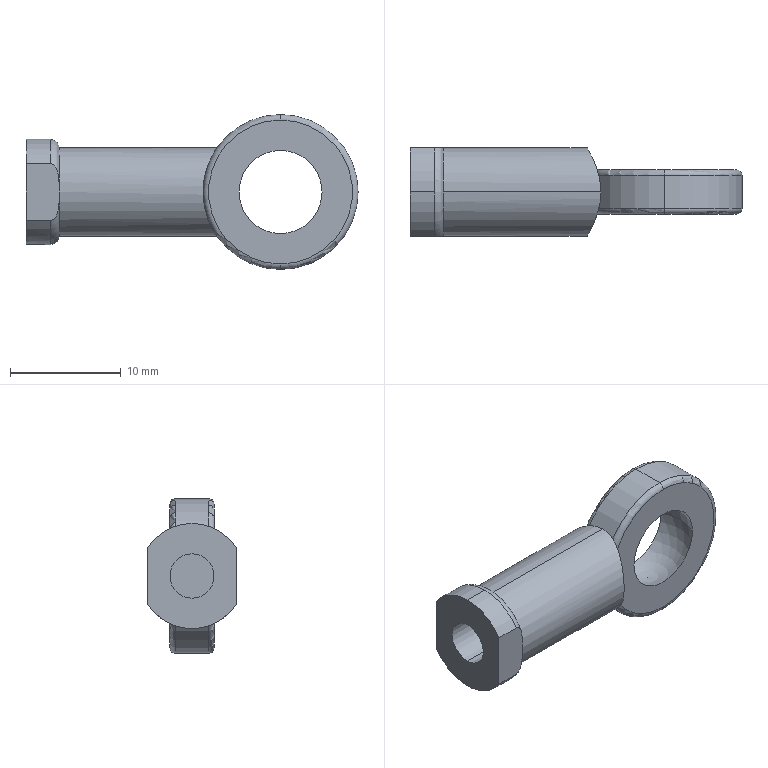Part | SolidWorks | features Fillet 3, ICE 3, Extrusion 1, RevCut 1 | 2 solids | 25 faces | box 30 x 8 x 14 mm | volume 1138 mm3 | cylinder 10 | torus 7 | plane 6 | sphere 2 | commonest cylinder face diameters 9.5 x3 14 x3 4 x2 8 x2
STEP:
#1=CARTESIAN_POINT('',(-3.75,0.,0.));
#2=VERTEX_POINT('',#1);
#3=CARTESIAN_POINT('',(3.75,0.,0.));
#4=VERTEX_POINT('',#3);
#5=CARTESIAN_POINT('',(0.,0.,0.));
#6=DIRECTION('',(0.,-1.,0.));
#7=DIRECTION('',(0.,0.,1.));
#8=AXIS2_PLACEMENT_3D('',#5,#6,#7);
#9=CIRCLE('',#8,3.75);
#10=EDGE_CURVE('',#2,#4,#9,.T.);
#11=ORIENTED_EDGE('',*,*,#10,.T.);
#12=CARTESIAN_POINT('',(3.75,4.,0.));
#13=VERTEX_POINT('',#12);
#14=CARTESIAN_POINT('',(0.,2.,0.));
#15=DIRECTION('',(0.,0.,1.));
#16=DIRECTION('',(1.,0.,0.));
#17=AXIS2_PLACEMENT_3D('',#14,#15,#16);
#18=CIRCLE('',#17,4.25);
#19=EDGE_CURVE('',#4,#13,#18,.T.);
#20=ORIENTED_EDGE('',*,*,#19,.T.);
#21=CARTESIAN_POINT('',(-3.75,4.,0.));
#22=VERTEX_POINT('',#21);
#23=CARTESIAN_POINT('',(0.,4.,0.));
#24=DIRECTION('',(0.,-1.,0.));
#25=DIRECTION('',(0.,0.,1.));
#26=AXIS2_PLACEMENT_3D('',#23,#24,#25);
#27=CIRCLE('',#26,3.75);
#28=EDGE_CURVE('',#22,#13,#27,.T.);
#29=ORIENTED_EDGE('',*,*,#28,.F.);
#30=CARTESIAN_POINT('',(0.,2.,0.));
#31=DIRECTION('',(0.,0.,-1.));
#32=DIRECTION('',(-1.,0.,0.));
#33=AXIS2_PLACEMENT_3D('',#30,#31,#32);
#34=CIRCLE('',#33,4.25);
#35=EDGE_CURVE('',#2,#22,#34,.T.);
#36=ORIENTED_EDGE('',*,*,#35,.F.);
#37=EDGE_LOOP('',(#11,#20,#29,#36));
#38=FACE_OUTER_BOUND('',#37,.T.);
#39=CARTESIAN_POINT('',(0.,2.,0.));
#40=DIRECTION('',(0.,0.,1.));
#41=DIRECTION('',(-1.,0.,0.));
#42=AXIS2_PLACEMENT_3D('',#39,#40,#41);
#43=SPHERICAL_SURFACE('',#42,4.25);
#44=ADVANCED_FACE('',(#38),#43,.F.);
#45=CARTESIAN_POINT('',(0.,3.5,-7.));
#46=VERTEX_POINT('',#45);
#47=CARTESIAN_POINT('',(0.,3.5,7.));
#48=VERTEX_POINT('',#47);
#49=CARTESIAN_POINT('',(0.,3.5,0.));
#50=DIRECTION('',(0.,-1.,0.));
#51=DIRECTION('',(0.,0.,1.));
#52=AXIS2_PLACEMENT_3D('',#49,#50,#51);
#53=CIRCLE('',#52,7.);
#54=EDGE_CURVE('',#46,#48,#53,.T.);
#55=ORIENTED_EDGE('',*,*,#54,.F.);
#56=CARTESIAN_POINT('',(0.,4.,-6.5));
#57=VERTEX_POINT('',#56);
#58=CARTESIAN_POINT('',(0.,3.5,-6.5));
#59=DIRECTION('',(1.,0.,0.));
#60=DIRECTION('',(0.,0.,-1.));
#61=AXIS2_PLACEMENT_3D('',#58,#59,#60);
#62=CIRCLE('',#61,0.5);
#63=EDGE_CURVE('',#46,#57,#62,.T.);
#64=ORIENTED_EDGE('',*,*,#63,.T.);
#65=CARTESIAN_POINT('',(0.,4.,6.5));
#66=VERTEX_POINT('',#65);
#67=CARTESIAN_POINT('',(0.,4.,0.));
#68=DIRECTION('',(0.,1.,0.));
#69=DIRECTION('',(0.,0.,1.));
#70=AXIS2_PLACEMENT_3D('',#67,#68,#69);
#71=CIRCLE('',#70,6.5);
#72=EDGE_CURVE('',#66,#57,#71,.T.);
#73=ORIENTED_EDGE('',*,*,#72,.F.);
#74=CARTESIAN_POINT('',(0.,3.5,6.5));
#75=DIRECTION('',(-1.,0.,0.));
#76=DIRECTION('',(0.,0.,1.));
#77=AXIS2_PLACEMENT_3D('',#74,#75,#76);
#78=CIRCLE('',#77,0.5);
#79=EDGE_CURVE('',#48,#66,#78,.T.);
#80=ORIENTED_EDGE('',*,*,#79,.F.);
#81=EDGE_LOOP('',(#55,#64,#73,#80));
#82=FACE_OUTER_BOUND('',#81,.T.);
#83=CARTESIAN_POINT('',(0.,3.5,0.));
#84=DIRECTION('',(0.,1.,0.));
#85=DIRECTION('',(0.,0.,1.));
#86=AXIS2_PLACEMENT_3D('',#83,#84,#85);
#87=TOROIDAL_SURFACE('',#86,6.5,0.5);
#88=ADVANCED_FACE('',(#82),#87,.T.);
#89=CARTESIAN_POINT('',(0.,0.,-6.5));
#90=VERTEX_POINT('',#89);
#91=CARTESIAN_POINT('',(0.,0.,6.5));
#92=VERTEX_POINT('',#91);
#93=CARTESIAN_POINT('',(0.,0.,0.));
#94=DIRECTION('',(0.,-1.,0.));
#95=DIRECTION('',(0.,0.,1.));
#96=AXIS2_PLACEMENT_3D('',#93,#94,#95);
#97=CIRCLE('',#96,6.5);
#98=EDGE_CURVE('',#90,#92,#97,.T.);
#99=ORIENTED_EDGE('',*,*,#98,.F.);
#100=CARTESIAN_POINT('',(0.,0.5,-7.));
#101=VERTEX_POINT('',#100);
#102=CARTESIAN_POINT('',(0.,0.5,-6.5));
#103=DIRECTION('',(1.,0.,0.));
#104=DIRECTION('',(0.,0.,-1.));
#105=AXIS2_PLACEMENT_3D('',#102,#103,#104);
#106=CIRCLE('',#105,0.5);
#107=EDGE_CURVE('',#90,#101,#106,.T.);
#108=ORIENTED_EDGE('',*,*,#107,.T.);
#109=CARTESIAN_POINT('',(0.,0.5,7.));
#110=VERTEX_POINT('',#109);
#111=CARTESIAN_POINT('',(0.,0.5,0.));
#112=DIRECTION('',(0.,1.,0.));
#113=DIRECTION('',(0.,0.,1.));
#114=AXIS2_PLACEMENT_3D('',#111,#112,#113);
#115=CIRCLE('',#114,7.);
#116=EDGE_CURVE('',#110,#101,#115,.T.);
#117=ORIENTED_EDGE('',*,*,#116,.F.);
#118=CARTESIAN_POINT('',(0.,0.5,6.5));
#119=DIRECTION('',(-1.,0.,0.));
#120=DIRECTION('',(0.,0.,1.));
#121=AXIS2_PLACEMENT_3D('',#118,#119,#120);
#122=CIRCLE('',#121,0.5);
#123=EDGE_CURVE('',#92,#110,#122,.T.);
#124=ORIENTED_EDGE('',*,*,#123,.F.);
#125=EDGE_LOOP('',(#99,#108,#117,#124));
#126=FACE_OUTER_BOUND('',#125,.T.);
#127=CARTESIAN_POINT('',(0.,0.5,0.));
#128=DIRECTION('',(0.,1.,0.));
#129=DIRECTION('',(0.,0.,1.));
#130=AXIS2_PLACEMENT_3D('',#127,#128,#129);
#131=TOROIDAL_SURFACE('',#130,6.5,0.5);
#132=ADVANCED_FACE('',(#126),#131,.T.);
#133=ORIENTED_EDGE('',*,*,#54,.T.);
#134=CARTESIAN_POINT('',(0.,4.,7.));
#135=DIRECTION('',(0.,-1.,0.));
#136=VECTOR('',#135,1000.);
#137=LINE('',#134,#136);
#138=EDGE_CURVE('',#48,#110,#137,.T.);
#139=ORIENTED_EDGE('',*,*,#138,.T.);
#140=ORIENTED_EDGE('',*,*,#116,.T.);
#141=CARTESIAN_POINT('',(0.,4.,-7.));
#142=DIRECTION('',(0.,-1.,0.));
#143=VECTOR('',#142,1000.);
#144=LINE('',#141,#143);
#145=EDGE_CURVE('',#46,#101,#144,.T.);
#146=ORIENTED_EDGE('',*,*,#145,.F.);
#147=EDGE_LOOP('',(#133,#139,#140,#146));
#148=FACE_OUTER_BOUND('',#147,.T.);
#149=CARTESIAN_POINT('',(0.,4.,0.));
#150=DIRECTION('',(0.,-1.,0.));
#151=DIRECTION('',(0.,0.,-1.));
#152=AXIS2_PLACEMENT_3D('',#149,#150,#151);
#153=CYLINDRICAL_SURFACE('',#152,7.);
#154=ADVANCED_FACE('',(#148),#153,.T.);
#155=ORIENTED_EDGE('',*,*,#28,.T.);
#156=CARTESIAN_POINT('',(0.,4.,0.));
#157=DIRECTION('',(0.,-1.,0.));
#158=DIRECTION('',(0.,0.,1.));
#159=AXIS2_PLACEMENT_3D('',#156,#157,#158);
#160=CIRCLE('',#159,3.75);
#161=EDGE_CURVE('',#13,#22,#160,.T.);
#162=ORIENTED_EDGE('',*,*,#161,.T.);
#163=EDGE_LOOP('',(#155,#162));
#164=FACE_BOUND('',#163,.T.);
#165=ORIENTED_EDGE('',*,*,#72,.T.);
#166=CARTESIAN_POINT('',(0.,4.,0.));
#167=DIRECTION('',(0.,1.,0.));
#168=DIRECTION('',(0.,0.,1.));
#169=AXIS2_PLACEMENT_3D('',#166,#167,#168);
#170=CIRCLE('',#169,6.5);
#171=EDGE_CURVE('',#57,#66,#170,.T.);
#172=ORIENTED_EDGE('',*,*,#171,.T.);
#173=EDGE_LOOP('',(#165,#172));
#174=FACE_OUTER_BOUND('',#173,.T.);
#175=CARTESIAN_POINT('',(0.,4.,0.));
#176=DIRECTION('',(0.,1.,0.));
#177=DIRECTION('',(0.,0.,1.));
#178=AXIS2_PLACEMENT_3D('',#175,#176,#177);
#179=PLANE('',#178);
#180=ADVANCED_FACE('',(#164,#174),#179,.T.);
#181=ORIENTED_EDGE('',*,*,#10,.F.);
#182=CARTESIAN_POINT('',(0.,0.,0.));
#183=DIRECTION('',(0.,-1.,0.));
#184=DIRECTION('',(0.,0.,1.));
#185=AXIS2_PLACEMENT_3D('',#182,#183,#184);
#186=CIRCLE('',#185,3.75);
#187=EDGE_CURVE('',#4,#2,#186,.T.);
#188=ORIENTED_EDGE('',*,*,#187,.F.);
#189=EDGE_LOOP('',(#181,#188));
#190=FACE_BOUND('',#189,.T.);
#191=CARTESIAN_POINT('',(0.,0.,0.));
#192=DIRECTION('',(0.,-1.,0.));
#193=DIRECTION('',(0.,0.,1.));
#194=AXIS2_PLACEMENT_3D('',#191,#192,#193);
#195=CIRCLE('',#194,6.5);
#196=EDGE_CURVE('',#92,#90,#195,.T.);
#197=ORIENTED_EDGE('',*,*,#196,.T.);
#198=ORIENTED_EDGE('',*,*,#98,.T.);
#199=EDGE_LOOP('',(#197,#198));
#200=FACE_OUTER_BOUND('',#199,.T.);
#201=CARTESIAN_POINT('',(0.,0.,0.));
#202=DIRECTION('',(0.,1.,0.));
#203=DIRECTION('',(0.,0.,1.));
#204=AXIS2_PLACEMENT_3D('',#201,#202,#203);
#205=PLANE('',#204);
#206=ADVANCED_FACE('',(#190,#200),#205,.F.);
#207=ORIENTED_EDGE('',*,*,#138,.F.);
#208=CARTESIAN_POINT('',(0.,3.5,0.));
#209=DIRECTION('',(0.,-1.,0.));
#210=DIRECTION('',(0.,0.,1.));
#211=AXIS2_PLACEMENT_3D('',#208,#209,#210);
#212=CIRCLE('',#211,7.);
#213=EDGE_CURVE('',#48,#46,#212,.T.);
#214=ORIENTED_EDGE('',*,*,#213,.T.);
#215=ORIENTED_EDGE('',*,*,#145,.T.);
#216=CARTESIAN_POINT('',(0.,0.5,0.));
#217=DIRECTION('',(0.,1.,0.));
#218=DIRECTION('',(0.,0.,1.));
#219=AXIS2_PLACEMENT_3D('',#216,#217,#218);
#220=CIRCLE('',#219,7.);
#221=EDGE_CURVE('',#101,#110,#220,.T.);
#222=ORIENTED_EDGE('',*,*,#221,.T.);
#223=EDGE_LOOP('',(#207,#214,#215,#222));
#224=FACE_OUTER_BOUND('',#223,.T.);
#225=CARTESIAN_POINT('',(0.,4.,0.));
#226=DIRECTION('',(0.,-1.,0.));
#227=DIRECTION('',(0.,0.,-1.));
#228=AXIS2_PLACEMENT_3D('',#225,#226,#227);
#229=CYLINDRICAL_SURFACE('',#228,7.);
#230=ADVANCED_FACE('',(#224),#229,.T.);
#231=ORIENTED_EDGE('',*,*,#107,.F.);
#232=ORIENTED_EDGE('',*,*,#196,.F.);
#233=ORIENTED_EDGE('',*,*,#123,.T.);
#234=ORIENTED_EDGE('',*,*,#221,.F.);
#235=EDGE_LOOP('',(#231,#232,#233,#234));
#236=FACE_OUTER_BOUND('',#235,.T.);
#237=CARTESIAN_POINT('',(0.,0.5,0.));
#238=DIRECTION('',(0.,1.,0.));
#239=DIRECTION('',(0.,0.,1.));
#240=AXIS2_PLACEMENT_3D('',#237,#238,#239);
#241=TOROIDAL_SURFACE('',#240,6.5,0.5);
#242=ADVANCED_FACE('',(#236),#241,.T.);
#243=ORIENTED_EDGE('',*,*,#63,.F.);
#244=ORIENTED_EDGE('',*,*,#213,.F.);
#245=ORIENTED_EDGE('',*,*,#79,.T.);
#246=ORIENTED_EDGE('',*,*,#171,.F.);
#247=EDGE_LOOP('',(#243,#244,#245,#246));
#248=FACE_OUTER_BOUND('',#247,.T.);
#249=CARTESIAN_POINT('',(0.,3.5,0.));
#250=DIRECTION('',(0.,1.,0.));
#251=DIRECTION('',(0.,0.,1.));
#252=AXIS2_PLACEMENT_3D('',#249,#250,#251);
#253=TOROIDAL_SURFACE('',#252,6.5,0.5);
#254=ADVANCED_FACE('',(#248),#253,.T.);
#255=ORIENTED_EDGE('',*,*,#19,.F.);
#256=ORIENTED_EDGE('',*,*,#187,.T.);
#257=ORIENTED_EDGE('',*,*,#35,.T.);
#258=ORIENTED_EDGE('',*,*,#161,.F.);
#259=EDGE_LOOP('',(#255,#256,#257,#258));
#260=FACE_OUTER_BOUND('',#259,.T.);
#261=CARTESIAN_POINT('',(0.,2.,0.));
#262=DIRECTION('',(0.,0.,1.));
#263=DIRECTION('',(-1.,0.,0.));
#264=AXIS2_PLACEMENT_3D('',#261,#262,#263);
#265=SPHERICAL_SURFACE('',#264,4.25);
#266=ADVANCED_FACE('',(#260),#265,.F.);
#267=CLOSED_SHELL('',(#44,#88,#132,#154,#180,#206,#230,#242,#254,#266));
#268=MANIFOLD_SOLID_BREP('',#267);
#269=CARTESIAN_POINT('',(-13.,2.,-2.));
#270=VERTEX_POINT('',#269);
#271=CARTESIAN_POINT('',(-13.,2.,2.));
#272=VERTEX_POINT('',#271);
#273=CARTESIAN_POINT('',(-13.,2.,0.));
#274=DIRECTION('',(-1.,0.,0.));
#275=DIRECTION('',(0.,0.,1.));
#276=AXIS2_PLACEMENT_3D('',#273,#274,#275);
#277=CIRCLE('',#276,2.);
#278=EDGE_CURVE('',#270,#272,#277,.T.);
#279=ORIENTED_EDGE('',*,*,#278,.F.);
#280=CARTESIAN_POINT('',(-23.,2.,-2.));
#281=VERTEX_POINT('',#280);
#282=CARTESIAN_POINT('',(-13.,2.,-2.));
#283=DIRECTION('',(-1.,0.,0.));
#284=VECTOR('',#283,1000.);
#285=LINE('',#282,#284);
#286=EDGE_CURVE('',#270,#281,#285,.T.);
#287=ORIENTED_EDGE('',*,*,#286,.T.);
#288=CARTESIAN_POINT('',(-23.,2.,2.));
#289=VERTEX_POINT('',#288);
#290=CARTESIAN_POINT('',(-23.,2.,0.));
#291=DIRECTION('',(-1.,0.,0.));
#292=DIRECTION('',(0.,0.,1.));
#293=AXIS2_PLACEMENT_3D('',#290,#291,#292);
#294=CIRCLE('',#293,2.);
#295=EDGE_CURVE('',#281,#289,#294,.T.);
#296=ORIENTED_EDGE('',*,*,#295,.T.);
#297=CARTESIAN_POINT('',(-13.,2.,2.));
#298=DIRECTION('',(-1.,0.,0.));
#299=VECTOR('',#298,1000.);
#300=LINE('',#297,#299);
#301=EDGE_CURVE('',#272,#289,#300,.T.);
#302=ORIENTED_EDGE('',*,*,#301,.F.);
#303=EDGE_LOOP('',(#279,#287,#296,#302));
#304=FACE_OUTER_BOUND('',#303,.T.);
#305=CARTESIAN_POINT('',(-13.,2.,0.));
#306=DIRECTION('',(-1.,0.,0.));
#307=DIRECTION('',(0.,0.,1.));
#308=AXIS2_PLACEMENT_3D('',#305,#306,#307);
#309=CYLINDRICAL_SURFACE('',#308,2.);
#310=ADVANCED_FACE('',(#304),#309,.F.);
#311=CARTESIAN_POINT('',(-20.798,2.,-4.75));
#312=VERTEX_POINT('',#311);
#313=CARTESIAN_POINT('',(-20.798,-2.,-2.562));
#314=VERTEX_POINT('',#313);
#315=CARTESIAN_POINT('',(-20.798,2.,0.));
#316=DIRECTION('',(-1.,0.,0.));
#317=DIRECTION('',(0.,0.,-1.));
#318=AXIS2_PLACEMENT_3D('',#315,#316,#317);
#319=CIRCLE('',#318,4.75);
#320=EDGE_CURVE('',#312,#314,#319,.T.);
#321=ORIENTED_EDGE('',*,*,#320,.F.);
#322=CARTESIAN_POINT('',(-20.,2.,-4.));
#323=VERTEX_POINT('',#322);
#324=CARTESIAN_POINT('',(-20.798,2.,-3.95));
#325=DIRECTION('',(0.,-1.,0.));
#326=DIRECTION('',(0.,0.,-1.));
#327=AXIS2_PLACEMENT_3D('',#324,#325,#326);
#328=CIRCLE('',#327,0.8);
#329=EDGE_CURVE('',#312,#323,#328,.T.);
#330=ORIENTED_EDGE('',*,*,#329,.T.);
#331=CARTESIAN_POINT('',(-20.,-2.,0.));
#332=VERTEX_POINT('',#331);
#333=CARTESIAN_POINT('',(-20.,2.,0.));
#334=DIRECTION('',(-1.,0.,0.));
#335=DIRECTION('',(0.,0.,1.));
#336=AXIS2_PLACEMENT_3D('',#333,#334,#335);
#337=CIRCLE('',#336,4.);
#338=EDGE_CURVE('',#323,#332,#337,.T.);
#339=ORIENTED_EDGE('',*,*,#338,.T.);
#340=CARTESIAN_POINT('',(-20.798,-2.,-2.562));
#341=CARTESIAN_POINT('',(-20.675,-2.,-2.562));
#342=CARTESIAN_POINT('',(-20.558,-2.,-2.506));
#343=CARTESIAN_POINT('',(-20.376,-2.,-2.346));
#344=CARTESIAN_POINT('',(-20.306,-2.,-2.243));
#345=CARTESIAN_POINT('',(-20.197,-2.,-2.027));
#346=CARTESIAN_POINT('',(-20.157,-2.,-1.911));
#347=CARTESIAN_POINT('',(-20.096,-2.,-1.678));
#348=CARTESIAN_POINT('',(-20.074,-2.,-1.56));
#349=CARTESIAN_POINT('',(-20.025,-2.,-1.204));
#350=CARTESIAN_POINT('',(-20.013,-2.,-0.9634));
#351=CARTESIAN_POINT('',(-20.001,-2.,-0.4818));
#352=CARTESIAN_POINT('',(-20.,-2.,-0.2409));
#353=CARTESIAN_POINT('',(-20.,-2.,0.));
#354=B_SPLINE_CURVE_WITH_KNOTS('',3,(#340,#341,#342,#343,#344,#345,#346,#347,#348,#349,#350,#351,#352,#353),.UNSPECIFIED.,.F.,.F.,(4,2,2,2,2,2,4),(0.,0.0003642,0.0007284,0.001093,0.001457,0.002185,0.002914),.UNSPECIFIED.);
#355=EDGE_CURVE('',#314,#332,#354,.T.);
#356=ORIENTED_EDGE('',*,*,#355,.F.);
#357=EDGE_LOOP('',(#321,#330,#339,#356));
#358=FACE_OUTER_BOUND('',#357,.T.);
#359=CARTESIAN_POINT('',(-20.798,2.,0.));
#360=DIRECTION('',(1.,0.,0.));
#361=DIRECTION('',(0.,0.,-1.));
#362=AXIS2_PLACEMENT_3D('',#359,#360,#361);
#363=TOROIDAL_SURFACE('',#362,3.95,0.8);
#364=ADVANCED_FACE('',(#358),#363,.T.);
#365=CARTESIAN_POINT('',(-20.798,-2.,2.562));
#366=VERTEX_POINT('',#365);
#367=CARTESIAN_POINT('',(-20.798,2.,4.75));
#368=VERTEX_POINT('',#367);
#369=CARTESIAN_POINT('',(-20.798,2.,0.));
#370=DIRECTION('',(-1.,0.,0.));
#371=DIRECTION('',(0.,0.,-1.));
#372=AXIS2_PLACEMENT_3D('',#369,#370,#371);
#373=CIRCLE('',#372,4.75);
#374=EDGE_CURVE('',#366,#368,#373,.T.);
#375=ORIENTED_EDGE('',*,*,#374,.T.);
#376=CARTESIAN_POINT('',(-23.,2.,4.75));
#377=VERTEX_POINT('',#376);
#378=CARTESIAN_POINT('',(-20.,2.,4.75));
#379=DIRECTION('',(-1.,0.,0.));
#380=VECTOR('',#379,1000.);
#381=LINE('',#378,#380);
#382=EDGE_CURVE('',#368,#377,#381,.T.);
#383=ORIENTED_EDGE('',*,*,#382,.T.);
#384=CARTESIAN_POINT('',(-23.,-2.,2.562));
#385=VERTEX_POINT('',#384);
#386=CARTESIAN_POINT('',(-23.,2.,0.));
#387=DIRECTION('',(-1.,0.,0.));
#388=DIRECTION('',(0.,0.,1.));
#389=AXIS2_PLACEMENT_3D('',#386,#387,#388);
#390=CIRCLE('',#389,4.75);
#391=EDGE_CURVE('',#385,#377,#390,.T.);
#392=ORIENTED_EDGE('',*,*,#391,.F.);
#393=CARTESIAN_POINT('',(-20.,-2.,2.562));
#394=DIRECTION('',(-1.,0.,0.));
#395=VECTOR('',#394,1000.);
#396=LINE('',#393,#395);
#397=EDGE_CURVE('',#366,#385,#396,.T.);
#398=ORIENTED_EDGE('',*,*,#397,.F.);
#399=EDGE_LOOP('',(#375,#383,#392,#398));
#400=FACE_OUTER_BOUND('',#399,.T.);
#401=CARTESIAN_POINT('',(-20.,2.,0.));
#402=DIRECTION('',(-1.,0.,0.));
#403=DIRECTION('',(0.,0.,1.));
#404=AXIS2_PLACEMENT_3D('',#401,#402,#403);
#405=CYLINDRICAL_SURFACE('',#404,4.75);
#406=ADVANCED_FACE('',(#400),#405,.T.);
#407=CARTESIAN_POINT('',(-20.,2.,4.));
#408=VERTEX_POINT('',#407);
#409=CARTESIAN_POINT('',(-20.,6.,0.));
#410=VERTEX_POINT('',#409);
#411=CARTESIAN_POINT('',(-20.,2.,0.));
#412=DIRECTION('',(-1.,0.,0.));
#413=DIRECTION('',(0.,0.,1.));
#414=AXIS2_PLACEMENT_3D('',#411,#412,#413);
#415=CIRCLE('',#414,4.);
#416=EDGE_CURVE('',#408,#410,#415,.T.);
#417=ORIENTED_EDGE('',*,*,#416,.F.);
#418=CARTESIAN_POINT('',(-5.745,2.,4.));
#419=VERTEX_POINT('',#418);
#420=CARTESIAN_POINT('',(-23.,2.,4.));
#421=DIRECTION('',(1.,0.,0.));
#422=VECTOR('',#421,1000.);
#423=LINE('',#420,#422);
#424=EDGE_CURVE('',#408,#419,#423,.T.);
#425=ORIENTED_EDGE('',*,*,#424,.T.);
#426=CARTESIAN_POINT('',(-5.745,2.,-4.));
#427=VERTEX_POINT('',#426);
#428=CARTESIAN_POINT('',(-5.745,2.,4.));
#429=CARTESIAN_POINT('',(-5.745,2.271,4.));
#430=CARTESIAN_POINT('',(-5.764,2.536,3.973));
#431=CARTESIAN_POINT('',(-5.835,3.055,3.868));
#432=CARTESIAN_POINT('',(-5.888,3.31,3.788));
#433=CARTESIAN_POINT('',(-6.075,4.031,3.485));
#434=CARTESIAN_POINT('',(-6.242,4.463,3.193));
#435=CARTESIAN_POINT('',(-6.481,5.005,2.652));
#436=CARTESIAN_POINT('',(-6.56,5.171,2.452));
#437=CARTESIAN_POINT('',(-6.705,5.46,2.024));
#438=CARTESIAN_POINT('',(-6.77,5.583,1.797));
#439=CARTESIAN_POINT('',(-6.879,5.786,1.317));
#440=CARTESIAN_POINT('',(-6.924,5.866,1.059));
#441=CARTESIAN_POINT('',(-6.984,5.972,0.539));
#442=CARTESIAN_POINT('',(-7.,6.,0.2747));
#443=CARTESIAN_POINT('',(-7.,6.,-0.1284));
#444=CARTESIAN_POINT('',(-6.996,5.994,-0.2644));
#445=CARTESIAN_POINT('',(-6.981,5.967,-0.5313));
#446=CARTESIAN_POINT('',(-6.97,5.947,-0.663));
#447=CARTESIAN_POINT('',(-6.925,5.868,-1.053));
#448=CARTESIAN_POINT('',(-6.881,5.789,-1.31));
#449=CARTESIAN_POINT('',(-6.771,5.584,-1.795));
#450=CARTESIAN_POINT('',(-6.705,5.46,-2.023));
#451=CARTESIAN_POINT('',(-6.56,5.17,-2.453));
#452=CARTESIAN_POINT('',(-6.481,5.005,-2.652));
#453=CARTESIAN_POINT('',(-6.322,4.644,-3.013));
#454=CARTESIAN_POINT('',(-6.24,4.445,-3.176));
#455=CARTESIAN_POINT('',(-6.085,4.017,-3.464));
#456=CARTESIAN_POINT('',(-6.013,3.791,-3.586));
#457=CARTESIAN_POINT('',(-5.919,3.432,-3.737));
#458=CARTESIAN_POINT('',(-5.891,3.31,-3.782));
#459=CARTESIAN_POINT('',(-5.84,3.057,-3.86));
#460=CARTESIAN_POINT('',(-5.817,2.927,-3.893));
#461=CARTESIAN_POINT('',(-5.764,2.536,-3.973));
#462=CARTESIAN_POINT('',(-5.745,2.27,-4.));
#463=CARTESIAN_POINT('',(-5.745,2.,-4.));
#464=B_SPLINE_CURVE_WITH_KNOTS('',3,(#428,#429,#430,#431,#432,#433,#434,#435,#436,#437,#438,#439,#440,#441,#442,#443,#444,#445,#446,#447,#448,#449,#450,#451,#452,#453,#454,#455,#456,#457,#458,#459,#460,#461,#462,#463),.UNSPECIFIED.,.F.,.F.,(4,2,2,2,2,2,2,2,2,2,2,2,2,2,2,2,2,4),(0.,0.0007996,0.001599,0.003198,0.003998,0.004798,0.005597,0.006397,0.006797,0.007197,0.007996,0.008796,0.009595,0.0104,0.01119,0.01159,0.01199,0.01279),.UNSPECIFIED.);
#465=EDGE_CURVE('',#419,#427,#464,.T.);
#466=ORIENTED_EDGE('',*,*,#465,.T.);
#467=CARTESIAN_POINT('',(-23.,2.,-4.));
#468=DIRECTION('',(1.,0.,0.));
#469=VECTOR('',#468,1000.);
#470=LINE('',#467,#469);
#471=EDGE_CURVE('',#323,#427,#470,.T.);
#472=ORIENTED_EDGE('',*,*,#471,.F.);
#473=CARTESIAN_POINT('',(-20.,2.,0.));
#474=DIRECTION('',(-1.,0.,0.));
#475=DIRECTION('',(0.,0.,1.));
#476=AXIS2_PLACEMENT_3D('',#473,#474,#475);
#477=CIRCLE('',#476,4.);
#478=EDGE_CURVE('',#410,#323,#477,.T.);
#479=ORIENTED_EDGE('',*,*,#478,.F.);
#480=EDGE_LOOP('',(#417,#425,#466,#472,#479));
#481=FACE_OUTER_BOUND('',#480,.T.);
#482=CARTESIAN_POINT('',(-23.,2.,0.));
#483=DIRECTION('',(1.,0.,0.));
#484=DIRECTION('',(0.,0.,-1.));
#485=AXIS2_PLACEMENT_3D('',#482,#483,#484);
#486=CYLINDRICAL_SURFACE('',#485,4.);
#487=ADVANCED_FACE('',(#481),#486,.T.);
#488=ORIENTED_EDGE('',*,*,#424,.F.);
#489=CARTESIAN_POINT('',(-20.,2.,0.));
#490=DIRECTION('',(-1.,0.,0.));
#491=DIRECTION('',(0.,0.,1.));
#492=AXIS2_PLACEMENT_3D('',#489,#490,#491);
#493=CIRCLE('',#492,4.);
#494=EDGE_CURVE('',#332,#408,#493,.T.);
#495=ORIENTED_EDGE('',*,*,#494,.F.);
#496=ORIENTED_EDGE('',*,*,#338,.F.);
#497=ORIENTED_EDGE('',*,*,#471,.T.);
#498=CARTESIAN_POINT('',(-5.745,2.,-4.));
#499=CARTESIAN_POINT('',(-5.745,1.73,-4.));
#500=CARTESIAN_POINT('',(-5.764,1.463,-3.973));
#501=CARTESIAN_POINT('',(-5.835,0.9435,-3.867));
#502=CARTESIAN_POINT('',(-5.888,0.6879,-3.788));
#503=CARTESIAN_POINT('',(-6.013,0.2078,-3.586));
#504=CARTESIAN_POINT('',(-6.086,-0.01982,-3.462));
#505=CARTESIAN_POINT('',(-6.241,-0.4485,-3.174));
#506=CARTESIAN_POINT('',(-6.322,-0.6451,-3.011));
#507=CARTESIAN_POINT('',(-6.482,-1.006,-2.651));
#508=CARTESIAN_POINT('',(-6.561,-1.172,-2.45));
#509=CARTESIAN_POINT('',(-6.705,-1.46,-2.023));
#510=CARTESIAN_POINT('',(-6.77,-1.583,-1.797));
#511=CARTESIAN_POINT('',(-6.88,-1.787,-1.315));
#512=CARTESIAN_POINT('',(-6.925,-1.867,-1.058));
#513=CARTESIAN_POINT('',(-6.984,-1.972,-0.5385));
#514=CARTESIAN_POINT('',(-7.,-2.,-0.2742));
#515=CARTESIAN_POINT('',(-7.,-2.,0.2646));
#516=CARTESIAN_POINT('',(-6.985,-1.973,0.5333));
#517=CARTESIAN_POINT('',(-6.925,-1.868,1.054));
#518=CARTESIAN_POINT('',(-6.881,-1.788,1.311));
#519=CARTESIAN_POINT('',(-6.771,-1.584,1.795));
#520=CARTESIAN_POINT('',(-6.705,-1.461,2.023));
#521=CARTESIAN_POINT('',(-6.56,-1.17,2.453));
#522=CARTESIAN_POINT('',(-6.481,-1.005,2.652));
#523=CARTESIAN_POINT('',(-6.322,-0.6439,3.012));
#524=CARTESIAN_POINT('',(-6.24,-0.4442,3.177));
#525=CARTESIAN_POINT('',(-6.085,-0.0172,3.464));
#526=CARTESIAN_POINT('',(-6.013,0.2084,3.586));
#527=CARTESIAN_POINT('',(-5.888,0.6864,3.787));
#528=CARTESIAN_POINT('',(-5.835,0.9424,3.867));
#529=CARTESIAN_POINT('',(-5.764,1.463,3.973));
#530=CARTESIAN_POINT('',(-5.745,1.73,4.));
#531=CARTESIAN_POINT('',(-5.745,2.,4.));
#532=B_SPLINE_CURVE_WITH_KNOTS('',3,(#498,#499,#500,#501,#502,#503,#504,#505,#506,#507,#508,#509,#510,#511,#512,#513,#514,#515,#516,#517,#518,#519,#520,#521,#522,#523,#524,#525,#526,#527,#528,#529,#530,#531),.UNSPECIFIED.,.F.,.F.,(4,2,2,2,2,2,2,2,2,2,2,2,2,2,2,2,4),(0.01279,0.01359,0.01439,0.01519,0.01599,0.01678,0.01758,0.01838,0.01918,0.01998,0.02077,0.02157,0.02237,0.02317,0.02397,0.02476,0.02556),.UNSPECIFIED.);
#533=EDGE_CURVE('',#427,#419,#532,.T.);
#534=ORIENTED_EDGE('',*,*,#533,.T.);
#535=EDGE_LOOP('',(#488,#495,#496,#497,#534));
#536=FACE_OUTER_BOUND('',#535,.T.);
#537=CARTESIAN_POINT('',(-23.,2.,0.));
#538=DIRECTION('',(1.,0.,0.));
#539=DIRECTION('',(0.,0.,-1.));
#540=AXIS2_PLACEMENT_3D('',#537,#538,#539);
#541=CYLINDRICAL_SURFACE('',#540,4.);
#542=ADVANCED_FACE('',(#536),#541,.T.);
#543=ORIENTED_EDGE('',*,*,#533,.F.);
#544=ORIENTED_EDGE('',*,*,#465,.F.);
#545=EDGE_LOOP('',(#543,#544));
#546=FACE_OUTER_BOUND('',#545,.T.);
#547=CARTESIAN_POINT('',(0.,4.,0.));
#548=DIRECTION('',(0.,-1.,0.));
#549=DIRECTION('',(0.,0.,-1.));
#550=AXIS2_PLACEMENT_3D('',#547,#548,#549);
#551=CYLINDRICAL_SURFACE('',#550,7.);
#552=ADVANCED_FACE('',(#546),#551,.F.);
#553=CARTESIAN_POINT('',(-23.,-2.,-2.562));
#554=VERTEX_POINT('',#553);
#555=CARTESIAN_POINT('',(-20.,-2.,-2.562));
#556=DIRECTION('',(-1.,0.,0.));
#557=VECTOR('',#556,1000.);
#558=LINE('',#555,#557);
#559=EDGE_CURVE('',#314,#554,#558,.T.);
#560=ORIENTED_EDGE('',*,*,#559,.F.);
#561=ORIENTED_EDGE('',*,*,#355,.T.);
#562=CARTESIAN_POINT('',(-20.,-2.,0.));
#563=CARTESIAN_POINT('',(-20.,-2.,0.2407));
#564=CARTESIAN_POINT('',(-20.001,-2.,0.4815));
#565=CARTESIAN_POINT('',(-20.013,-2.,0.9623));
#566=CARTESIAN_POINT('',(-20.025,-2.,1.202));
#567=CARTESIAN_POINT('',(-20.074,-2.,1.561));
#568=CARTESIAN_POINT('',(-20.096,-2.,1.681));
#569=CARTESIAN_POINT('',(-20.158,-2.,1.914));
#570=CARTESIAN_POINT('',(-20.199,-2.,2.03));
#571=CARTESIAN_POINT('',(-20.307,-2.,2.244));
#572=CARTESIAN_POINT('',(-20.376,-2.,2.346));
#573=CARTESIAN_POINT('',(-20.559,-2.,2.506));
#574=CARTESIAN_POINT('',(-20.675,-2.,2.562));
#575=CARTESIAN_POINT('',(-20.798,-2.,2.562));
#576=B_SPLINE_CURVE_WITH_KNOTS('',3,(#562,#563,#564,#565,#566,#567,#568,#569,#570,#571,#572,#573,#574,#575),.UNSPECIFIED.,.F.,.F.,(4,2,2,2,2,2,4),(0.,0.0007213,0.001443,0.001803,0.002164,0.002524,0.002885),.UNSPECIFIED.);
#577=EDGE_CURVE('',#332,#366,#576,.T.);
#578=ORIENTED_EDGE('',*,*,#577,.T.);
#579=ORIENTED_EDGE('',*,*,#397,.T.);
#580=CARTESIAN_POINT('',(-23.,-2.,2.562));
#581=DIRECTION('',(0.,0.,1.));
#582=VECTOR('',#581,1000.);
#583=LINE('',#580,#582);
#584=EDGE_CURVE('',#554,#385,#583,.T.);
#585=ORIENTED_EDGE('',*,*,#584,.F.);
#586=EDGE_LOOP('',(#560,#561,#578,#579,#585));
#587=FACE_OUTER_BOUND('',#586,.T.);
#588=CARTESIAN_POINT('',(-20.,-2.,2.562));
#589=DIRECTION('',(0.,-1.,0.));
#590=DIRECTION('',(0.,0.,-1.));
#591=AXIS2_PLACEMENT_3D('',#588,#589,#590);
#592=PLANE('',#591);
#593=ADVANCED_FACE('',(#587),#592,.T.);
#594=CARTESIAN_POINT('',(-20.798,6.,2.562));
#595=VERTEX_POINT('',#594);
#596=CARTESIAN_POINT('',(-20.798,6.,2.562));
#597=CARTESIAN_POINT('',(-20.675,6.,2.562));
#598=CARTESIAN_POINT('',(-20.558,6.,2.506));
#599=CARTESIAN_POINT('',(-20.376,6.,2.346));
#600=CARTESIAN_POINT('',(-20.306,6.,2.243));
#601=CARTESIAN_POINT('',(-20.197,6.,2.027));
#602=CARTESIAN_POINT('',(-20.157,6.,1.911));
#603=CARTESIAN_POINT('',(-20.096,6.,1.678));
#604=CARTESIAN_POINT('',(-20.074,6.,1.56));
#605=CARTESIAN_POINT('',(-20.025,6.,1.204));
#606=CARTESIAN_POINT('',(-20.013,6.,0.9634));
#607=CARTESIAN_POINT('',(-20.001,6.,0.4818));
#608=CARTESIAN_POINT('',(-20.,6.,0.2409));
#609=CARTESIAN_POINT('',(-20.,6.,0.));
#610=B_SPLINE_CURVE_WITH_KNOTS('',3,(#596,#597,#598,#599,#600,#601,#602,#603,#604,#605,#606,#607,#608,#609),.UNSPECIFIED.,.F.,.F.,(4,2,2,2,2,2,4),(0.,0.0003642,0.0007284,0.001093,0.001457,0.002185,0.002914),.UNSPECIFIED.);
#611=EDGE_CURVE('',#595,#410,#610,.T.);
#612=ORIENTED_EDGE('',*,*,#611,.T.);
#613=CARTESIAN_POINT('',(-20.798,6.,-2.562));
#614=VERTEX_POINT('',#613);
#615=CARTESIAN_POINT('',(-20.,6.,0.));
#616=CARTESIAN_POINT('',(-20.,6.,-0.2407));
#617=CARTESIAN_POINT('',(-20.001,6.,-0.4815));
#618=CARTESIAN_POINT('',(-20.013,6.,-0.9623));
#619=CARTESIAN_POINT('',(-20.025,6.,-1.202));
#620=CARTESIAN_POINT('',(-20.074,6.,-1.561));
#621=CARTESIAN_POINT('',(-20.096,6.,-1.681));
#622=CARTESIAN_POINT('',(-20.158,6.,-1.914));
#623=CARTESIAN_POINT('',(-20.199,6.,-2.03));
#624=CARTESIAN_POINT('',(-20.307,6.,-2.244));
#625=CARTESIAN_POINT('',(-20.376,6.,-2.346));
#626=CARTESIAN_POINT('',(-20.559,6.,-2.506));
#627=CARTESIAN_POINT('',(-20.675,6.,-2.562));
#628=CARTESIAN_POINT('',(-20.798,6.,-2.562));
#629=B_SPLINE_CURVE_WITH_KNOTS('',3,(#615,#616,#617,#618,#619,#620,#621,#622,#623,#624,#625,#626,#627,#628),.UNSPECIFIED.,.F.,.F.,(4,2,2,2,2,2,4),(0.,0.0007213,0.001443,0.001803,0.002164,0.002524,0.002885),.UNSPECIFIED.);
#630=EDGE_CURVE('',#410,#614,#629,.T.);
#631=ORIENTED_EDGE('',*,*,#630,.T.);
#632=CARTESIAN_POINT('',(-23.,6.,-2.562));
#633=VERTEX_POINT('',#632);
#634=CARTESIAN_POINT('',(-20.,6.,-2.562));
#635=DIRECTION('',(-1.,0.,0.));
#636=VECTOR('',#635,1000.);
#637=LINE('',#634,#636);
#638=EDGE_CURVE('',#614,#633,#637,.T.);
#639=ORIENTED_EDGE('',*,*,#638,.T.);
#640=CARTESIAN_POINT('',(-23.,6.,2.562));
#641=VERTEX_POINT('',#640);
#642=CARTESIAN_POINT('',(-23.,6.,2.562));
#643=DIRECTION('',(0.,0.,-1.));
#644=VECTOR('',#643,1000.);
#645=LINE('',#642,#644);
#646=EDGE_CURVE('',#641,#633,#645,.T.);
#647=ORIENTED_EDGE('',*,*,#646,.F.);
#648=CARTESIAN_POINT('',(-20.,6.,2.562));
#649=DIRECTION('',(-1.,0.,0.));
#650=VECTOR('',#649,1000.);
#651=LINE('',#648,#650);
#652=EDGE_CURVE('',#595,#641,#651,.T.);
#653=ORIENTED_EDGE('',*,*,#652,.F.);
#654=EDGE_LOOP('',(#612,#631,#639,#647,#653));
#655=FACE_OUTER_BOUND('',#654,.T.);
#656=CARTESIAN_POINT('',(-20.,6.,2.562));
#657=DIRECTION('',(0.,1.,0.));
#658=DIRECTION('',(0.,0.,1.));
#659=AXIS2_PLACEMENT_3D('',#656,#657,#658);
#660=PLANE('',#659);
#661=ADVANCED_FACE('',(#655),#660,.T.);
#662=ORIENTED_EDGE('',*,*,#382,.F.);
#663=CARTESIAN_POINT('',(-20.798,2.,0.));
#664=DIRECTION('',(-1.,0.,0.));
#665=DIRECTION('',(0.,0.,-1.));
#666=AXIS2_PLACEMENT_3D('',#663,#664,#665);
#667=CIRCLE('',#666,4.75);
#668=EDGE_CURVE('',#368,#595,#667,.T.);
#669=ORIENTED_EDGE('',*,*,#668,.T.);
#670=ORIENTED_EDGE('',*,*,#652,.T.);
#671=CARTESIAN_POINT('',(-23.,2.,0.));
#672=DIRECTION('',(-1.,0.,0.));
#673=DIRECTION('',(0.,0.,1.));
#674=AXIS2_PLACEMENT_3D('',#671,#672,#673);
#675=CIRCLE('',#674,4.75);
#676=EDGE_CURVE('',#377,#641,#675,.T.);
#677=ORIENTED_EDGE('',*,*,#676,.F.);
#678=EDGE_LOOP('',(#662,#669,#670,#677));
#679=FACE_OUTER_BOUND('',#678,.T.);
#680=CARTESIAN_POINT('',(-20.,2.,0.));
#681=DIRECTION('',(-1.,0.,0.));
#682=DIRECTION('',(0.,0.,1.));
#683=AXIS2_PLACEMENT_3D('',#680,#681,#682);
#684=CYLINDRICAL_SURFACE('',#683,4.75);
#685=ADVANCED_FACE('',(#679),#684,.T.);
#686=ORIENTED_EDGE('',*,*,#638,.F.);
#687=CARTESIAN_POINT('',(-20.798,2.,0.));
#688=DIRECTION('',(-1.,0.,0.));
#689=DIRECTION('',(0.,0.,-1.));
#690=AXIS2_PLACEMENT_3D('',#687,#688,#689);
#691=CIRCLE('',#690,4.75);
#692=EDGE_CURVE('',#614,#312,#691,.T.);
#693=ORIENTED_EDGE('',*,*,#692,.T.);
#694=ORIENTED_EDGE('',*,*,#320,.T.);
#695=ORIENTED_EDGE('',*,*,#559,.T.);
#696=CARTESIAN_POINT('',(-23.,2.,0.));
#697=DIRECTION('',(-1.,0.,0.));
#698=DIRECTION('',(0.,0.,1.));
#699=AXIS2_PLACEMENT_3D('',#696,#697,#698);
#700=CIRCLE('',#699,4.75);
#701=EDGE_CURVE('',#633,#554,#700,.T.);
#702=ORIENTED_EDGE('',*,*,#701,.F.);
#703=EDGE_LOOP('',(#686,#693,#694,#695,#702));
#704=FACE_OUTER_BOUND('',#703,.T.);
#705=CARTESIAN_POINT('',(-20.,2.,0.));
#706=DIRECTION('',(-1.,0.,0.));
#707=DIRECTION('',(0.,0.,1.));
#708=AXIS2_PLACEMENT_3D('',#705,#706,#707);
#709=CYLINDRICAL_SURFACE('',#708,4.75);
#710=ADVANCED_FACE('',(#704),#709,.T.);
#711=CARTESIAN_POINT('',(-23.,2.,0.));
#712=DIRECTION('',(-1.,0.,0.));
#713=DIRECTION('',(0.,0.,1.));
#714=AXIS2_PLACEMENT_3D('',#711,#712,#713);
#715=CIRCLE('',#714,2.);
#716=EDGE_CURVE('',#289,#281,#715,.T.);
#717=ORIENTED_EDGE('',*,*,#716,.F.);
#718=ORIENTED_EDGE('',*,*,#295,.F.);
#719=EDGE_LOOP('',(#717,#718));
#720=FACE_BOUND('',#719,.T.);
#721=ORIENTED_EDGE('',*,*,#391,.T.);
#722=ORIENTED_EDGE('',*,*,#676,.T.);
#723=ORIENTED_EDGE('',*,*,#646,.T.);
#724=ORIENTED_EDGE('',*,*,#701,.T.);
#725=ORIENTED_EDGE('',*,*,#584,.T.);
#726=EDGE_LOOP('',(#721,#722,#723,#724,#725));
#727=FACE_OUTER_BOUND('',#726,.T.);
#728=CARTESIAN_POINT('',(-23.,2.,0.));
#729=DIRECTION('',(-1.,0.,0.));
#730=DIRECTION('',(0.,0.,1.));
#731=AXIS2_PLACEMENT_3D('',#728,#729,#730);
#732=PLANE('',#731);
#733=ADVANCED_FACE('',(#720,#727),#732,.T.);
#734=ORIENTED_EDGE('',*,*,#329,.F.);
#735=ORIENTED_EDGE('',*,*,#692,.F.);
#736=ORIENTED_EDGE('',*,*,#630,.F.);
#737=ORIENTED_EDGE('',*,*,#478,.T.);
#738=EDGE_LOOP('',(#734,#735,#736,#737));
#739=FACE_OUTER_BOUND('',#738,.T.);
#740=CARTESIAN_POINT('',(-20.798,2.,0.));
#741=DIRECTION('',(1.,0.,0.));
#742=DIRECTION('',(0.,0.,-1.));
#743=AXIS2_PLACEMENT_3D('',#740,#741,#742);
#744=TOROIDAL_SURFACE('',#743,3.95,0.8);
#745=ADVANCED_FACE('',(#739),#744,.T.);
#746=ORIENTED_EDGE('',*,*,#577,.F.);
#747=ORIENTED_EDGE('',*,*,#494,.T.);
#748=ORIENTED_EDGE('',*,*,#416,.T.);
#749=ORIENTED_EDGE('',*,*,#611,.F.);
#750=ORIENTED_EDGE('',*,*,#668,.F.);
#751=ORIENTED_EDGE('',*,*,#374,.F.);
#752=EDGE_LOOP('',(#746,#747,#748,#749,#750,#751));
#753=FACE_OUTER_BOUND('',#752,.T.);
#754=CARTESIAN_POINT('',(-20.798,2.,0.));
#755=DIRECTION('',(1.,0.,0.));
#756=DIRECTION('',(0.,0.,-1.));
#757=AXIS2_PLACEMENT_3D('',#754,#755,#756);
#758=TOROIDAL_SURFACE('',#757,3.95,0.8);
#759=ADVANCED_FACE('',(#753),#758,.T.);
#760=ORIENTED_EDGE('',*,*,#286,.F.);
#761=CARTESIAN_POINT('',(-13.,2.,0.));
#762=DIRECTION('',(-1.,0.,0.));
#763=DIRECTION('',(0.,0.,1.));
#764=AXIS2_PLACEMENT_3D('',#761,#762,#763);
#765=CIRCLE('',#764,2.);
#766=EDGE_CURVE('',#272,#270,#765,.T.);
#767=ORIENTED_EDGE('',*,*,#766,.F.);
#768=ORIENTED_EDGE('',*,*,#301,.T.);
#769=ORIENTED_EDGE('',*,*,#716,.T.);
#770=EDGE_LOOP('',(#760,#767,#768,#769));
#771=FACE_OUTER_BOUND('',#770,.T.);
#772=CARTESIAN_POINT('',(-13.,2.,0.));
#773=DIRECTION('',(-1.,0.,0.));
#774=DIRECTION('',(0.,0.,1.));
#775=AXIS2_PLACEMENT_3D('',#772,#773,#774);
#776=CYLINDRICAL_SURFACE('',#775,2.);
#777=ADVANCED_FACE('',(#771),#776,.F.);
#778=ORIENTED_EDGE('',*,*,#766,.T.);
#779=ORIENTED_EDGE('',*,*,#278,.T.);
#780=EDGE_LOOP('',(#778,#779));
#781=FACE_OUTER_BOUND('',#780,.T.);
#782=CARTESIAN_POINT('',(-13.,2.,0.));
#783=DIRECTION('',(-1.,0.,0.));
#784=DIRECTION('',(0.,0.,1.));
#785=AXIS2_PLACEMENT_3D('',#782,#783,#784);
#786=PLANE('',#785);
#787=ADVANCED_FACE('',(#781),#786,.T.);
#788=CLOSED_SHELL('',(#310,#364,#406,#487,#542,#552,#593,#661,#685,#710,#733,#745,#759,#777,#787));
#789=MANIFOLD_SOLID_BREP('',#788);
#790=CARTESIAN_POINT('',(0.,0.,0.));
#791=DIRECTION('',(0.,0.,1.));
#792=DIRECTION('',(1.,0.,0.));
#793=AXIS2_PLACEMENT_3D('',#790,#791,#792);
#794=(LENGTH_UNIT()NAMED_UNIT(*)SI_UNIT(.MILLI.,.METRE.));
#795=UNCERTAINTY_MEASURE_WITH_UNIT(LENGTH_MEASURE(0.00001),#794,'','');
#796=(NAMED_UNIT(*)PLANE_ANGLE_UNIT()SI_UNIT($,.RADIAN.));
#797=(NAMED_UNIT(*)SI_UNIT($,.STERADIAN.)SOLID_ANGLE_UNIT());
#798=(GEOMETRIC_REPRESENTATION_CONTEXT(3)GLOBAL_UNCERTAINTY_ASSIGNED_CONTEXT((#795))GLOBAL_UNIT_ASSIGNED_CONTEXT((#794,#796,#797))REPRESENTATION_CONTEXT('',''));
#799=ADVANCED_BREP_SHAPE_REPRESENTATION('',(#268,#789,#793),#798);